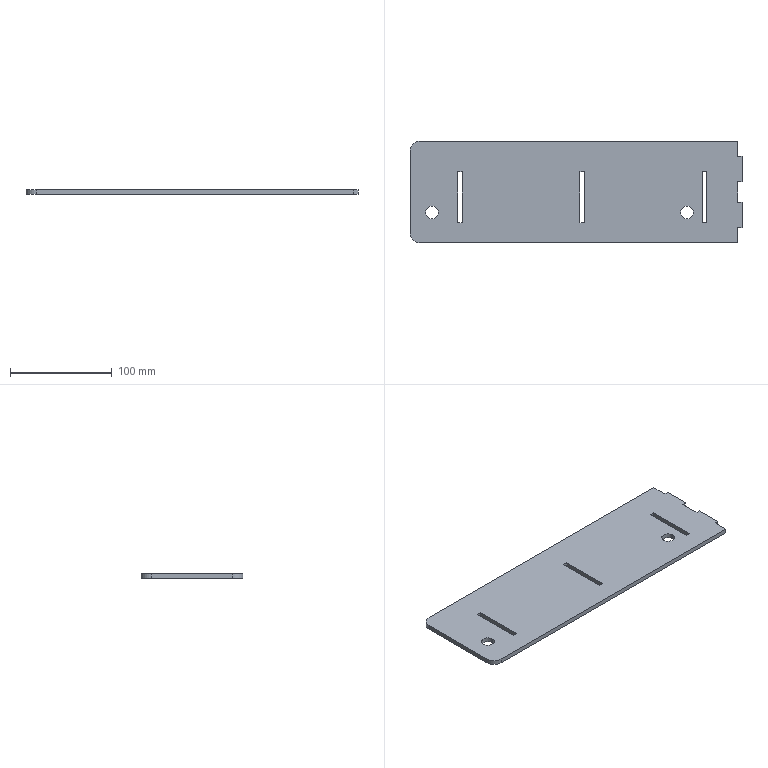Part | SolidWorks | features Fillet 1, FlatPattern 1, SMBaseFlange 1, SheetMetal 1 | 1 solid | 32 faces | box 325.679 x 100 x 4.5 mm | volume 141321 mm3 | plane 26 | cylinder 6 | commonest cylinder face diameters 12.5 x4 20 x2
STEP:
#1=CARTESIAN_POINT('',(173.75,-25.,4.5));
#2=VERTEX_POINT('',#1);
#3=CARTESIAN_POINT('',(186.25,-25.,4.5));
#4=VERTEX_POINT('',#3);
#5=CARTESIAN_POINT('',(180.,-25.,4.5));
#6=DIRECTION('',(0.,0.,1.));
#7=DIRECTION('',(1.,0.,0.));
#8=AXIS2_PLACEMENT_3D('',#5,#6,#7);
#9=CIRCLE('',#8,6.25);
#10=EDGE_CURVE('',#2,#4,#9,.T.);
#11=ORIENTED_EDGE('',*,*,#10,.T.);
#12=CARTESIAN_POINT('',(186.25,-25.,0.));
#13=VERTEX_POINT('',#12);
#14=CARTESIAN_POINT('',(186.25,-25.,4.5));
#15=DIRECTION('',(0.,0.,-1.));
#16=VECTOR('',#15,1000.);
#17=LINE('',#14,#16);
#18=EDGE_CURVE('',#4,#13,#17,.T.);
#19=ORIENTED_EDGE('',*,*,#18,.T.);
#20=CARTESIAN_POINT('',(173.75,-25.,0.));
#21=VERTEX_POINT('',#20);
#22=CARTESIAN_POINT('',(180.,-25.,0.));
#23=DIRECTION('',(0.,0.,1.));
#24=DIRECTION('',(1.,0.,0.));
#25=AXIS2_PLACEMENT_3D('',#22,#23,#24);
#26=CIRCLE('',#25,6.25);
#27=EDGE_CURVE('',#21,#13,#26,.T.);
#28=ORIENTED_EDGE('',*,*,#27,.F.);
#29=CARTESIAN_POINT('',(173.75,-25.,4.5));
#30=DIRECTION('',(0.,0.,-1.));
#31=VECTOR('',#30,1000.);
#32=LINE('',#29,#31);
#33=EDGE_CURVE('',#2,#21,#32,.T.);
#34=ORIENTED_EDGE('',*,*,#33,.F.);
#35=EDGE_LOOP('',(#11,#19,#28,#34));
#36=FACE_OUTER_BOUND('',#35,.T.);
#37=CARTESIAN_POINT('',(180.,-25.,4.5));
#38=DIRECTION('',(0.,0.,-1.));
#39=DIRECTION('',(-1.,0.,0.));
#40=AXIS2_PLACEMENT_3D('',#37,#38,#39);
#41=CYLINDRICAL_SURFACE('',#40,6.25);
#42=ADVANCED_FACE('',(#36),#41,.F.);
#43=CARTESIAN_POINT('',(-76.25,-25.,4.5));
#44=VERTEX_POINT('',#43);
#45=CARTESIAN_POINT('',(-63.75,-25.,4.5));
#46=VERTEX_POINT('',#45);
#47=CARTESIAN_POINT('',(-70.,-25.,4.5));
#48=DIRECTION('',(0.,0.,1.));
#49=DIRECTION('',(1.,0.,0.));
#50=AXIS2_PLACEMENT_3D('',#47,#48,#49);
#51=CIRCLE('',#50,6.25);
#52=EDGE_CURVE('',#44,#46,#51,.T.);
#53=ORIENTED_EDGE('',*,*,#52,.T.);
#54=CARTESIAN_POINT('',(-63.75,-25.,0.));
#55=VERTEX_POINT('',#54);
#56=CARTESIAN_POINT('',(-63.75,-25.,4.5));
#57=DIRECTION('',(0.,0.,-1.));
#58=VECTOR('',#57,1000.);
#59=LINE('',#56,#58);
#60=EDGE_CURVE('',#46,#55,#59,.T.);
#61=ORIENTED_EDGE('',*,*,#60,.T.);
#62=CARTESIAN_POINT('',(-76.25,-25.,0.));
#63=VERTEX_POINT('',#62);
#64=CARTESIAN_POINT('',(-70.,-25.,0.));
#65=DIRECTION('',(0.,0.,1.));
#66=DIRECTION('',(1.,0.,0.));
#67=AXIS2_PLACEMENT_3D('',#64,#65,#66);
#68=CIRCLE('',#67,6.25);
#69=EDGE_CURVE('',#63,#55,#68,.T.);
#70=ORIENTED_EDGE('',*,*,#69,.F.);
#71=CARTESIAN_POINT('',(-76.25,-25.,4.5));
#72=DIRECTION('',(0.,0.,-1.));
#73=VECTOR('',#72,1000.);
#74=LINE('',#71,#73);
#75=EDGE_CURVE('',#44,#63,#74,.T.);
#76=ORIENTED_EDGE('',*,*,#75,.F.);
#77=EDGE_LOOP('',(#53,#61,#70,#76));
#78=FACE_OUTER_BOUND('',#77,.T.);
#79=CARTESIAN_POINT('',(-70.,-25.,4.5));
#80=DIRECTION('',(0.,0.,-1.));
#81=DIRECTION('',(-1.,0.,0.));
#82=AXIS2_PLACEMENT_3D('',#79,#80,#81);
#83=CYLINDRICAL_SURFACE('',#82,6.25);
#84=ADVANCED_FACE('',(#78),#83,.F.);
#85=CARTESIAN_POINT('',(79.5,-35.,4.5));
#86=VERTEX_POINT('',#85);
#87=CARTESIAN_POINT('',(79.5,15.,4.5));
#88=VERTEX_POINT('',#87);
#89=CARTESIAN_POINT('',(79.5,-35.,4.5));
#90=DIRECTION('',(0.,1.,0.));
#91=VECTOR('',#90,1000.);
#92=LINE('',#89,#91);
#93=EDGE_CURVE('',#86,#88,#92,.T.);
#94=ORIENTED_EDGE('',*,*,#93,.F.);
#95=CARTESIAN_POINT('',(75.,-35.,4.5));
#96=VERTEX_POINT('',#95);
#97=CARTESIAN_POINT('',(79.5,-35.,4.5));
#98=DIRECTION('',(1.,0.,0.));
#99=VECTOR('',#98,1000.);
#100=LINE('',#97,#99);
#101=EDGE_CURVE('',#96,#86,#100,.T.);
#102=ORIENTED_EDGE('',*,*,#101,.F.);
#103=CARTESIAN_POINT('',(75.,15.,4.5));
#104=VERTEX_POINT('',#103);
#105=CARTESIAN_POINT('',(75.,-35.,4.5));
#106=DIRECTION('',(0.,-1.,0.));
#107=VECTOR('',#106,1000.);
#108=LINE('',#105,#107);
#109=EDGE_CURVE('',#104,#96,#108,.T.);
#110=ORIENTED_EDGE('',*,*,#109,.F.);
#111=CARTESIAN_POINT('',(79.5,15.,4.5));
#112=DIRECTION('',(-1.,0.,0.));
#113=VECTOR('',#112,1000.);
#114=LINE('',#111,#113);
#115=EDGE_CURVE('',#88,#104,#114,.T.);
#116=ORIENTED_EDGE('',*,*,#115,.F.);
#117=EDGE_LOOP('',(#94,#102,#110,#116));
#118=FACE_BOUND('',#117,.T.);
#119=CARTESIAN_POINT('',(-91.679,35.,4.5));
#120=VERTEX_POINT('',#119);
#121=CARTESIAN_POINT('',(-91.679,-45.,4.5));
#122=VERTEX_POINT('',#121);
#123=CARTESIAN_POINT('',(-91.679,-55.,4.5));
#124=DIRECTION('',(0.,-1.,0.));
#125=VECTOR('',#124,1000.);
#126=LINE('',#123,#125);
#127=EDGE_CURVE('',#120,#122,#126,.T.);
#128=ORIENTED_EDGE('',*,*,#127,.T.);
#129=CARTESIAN_POINT('',(-81.679,-55.,4.5));
#130=VERTEX_POINT('',#129);
#131=CARTESIAN_POINT('',(-81.679,-45.,4.5));
#132=DIRECTION('',(0.,0.,1.));
#133=DIRECTION('',(-1.,0.,0.));
#134=AXIS2_PLACEMENT_3D('',#131,#132,#133);
#135=CIRCLE('',#134,10.);
#136=EDGE_CURVE('',#122,#130,#135,.T.);
#137=ORIENTED_EDGE('',*,*,#136,.T.);
#138=CARTESIAN_POINT('',(230.,-55.,4.5));
#139=VERTEX_POINT('',#138);
#140=CARTESIAN_POINT('',(230.,-55.,4.5));
#141=DIRECTION('',(1.,0.,0.));
#142=VECTOR('',#141,1000.);
#143=LINE('',#140,#142);
#144=EDGE_CURVE('',#130,#139,#143,.T.);
#145=ORIENTED_EDGE('',*,*,#144,.T.);
#146=CARTESIAN_POINT('',(230.,-40.,4.5));
#147=VERTEX_POINT('',#146);
#148=CARTESIAN_POINT('',(230.,-40.,4.5));
#149=DIRECTION('',(0.,1.,0.));
#150=VECTOR('',#149,1000.);
#151=LINE('',#148,#150);
#152=EDGE_CURVE('',#139,#147,#151,.T.);
#153=ORIENTED_EDGE('',*,*,#152,.T.);
#154=CARTESIAN_POINT('',(234.,-40.,4.5));
#155=VERTEX_POINT('',#154);
#156=CARTESIAN_POINT('',(234.,-40.,4.5));
#157=DIRECTION('',(1.,0.,0.));
#158=VECTOR('',#157,1000.);
#159=LINE('',#156,#158);
#160=EDGE_CURVE('',#147,#155,#159,.T.);
#161=ORIENTED_EDGE('',*,*,#160,.T.);
#162=CARTESIAN_POINT('',(234.,-15.,4.5));
#163=VERTEX_POINT('',#162);
#164=CARTESIAN_POINT('',(234.,-15.,4.5));
#165=DIRECTION('',(0.,1.,0.));
#166=VECTOR('',#165,1000.);
#167=LINE('',#164,#166);
#168=EDGE_CURVE('',#155,#163,#167,.T.);
#169=ORIENTED_EDGE('',*,*,#168,.T.);
#170=CARTESIAN_POINT('',(230.,-15.,4.5));
#171=VERTEX_POINT('',#170);
#172=CARTESIAN_POINT('',(230.,-15.,4.5));
#173=DIRECTION('',(-1.,0.,0.));
#174=VECTOR('',#173,1000.);
#175=LINE('',#172,#174);
#176=EDGE_CURVE('',#163,#171,#175,.T.);
#177=ORIENTED_EDGE('',*,*,#176,.T.);
#178=CARTESIAN_POINT('',(230.,5.,4.5));
#179=VERTEX_POINT('',#178);
#180=CARTESIAN_POINT('',(230.,5.,4.5));
#181=DIRECTION('',(0.,1.,0.));
#182=VECTOR('',#181,1000.);
#183=LINE('',#180,#182);
#184=EDGE_CURVE('',#171,#179,#183,.T.);
#185=ORIENTED_EDGE('',*,*,#184,.T.);
#186=CARTESIAN_POINT('',(234.,5.,4.5));
#187=VERTEX_POINT('',#186);
#188=CARTESIAN_POINT('',(234.,5.,4.5));
#189=DIRECTION('',(1.,0.,0.));
#190=VECTOR('',#189,1000.);
#191=LINE('',#188,#190);
#192=EDGE_CURVE('',#179,#187,#191,.T.);
#193=ORIENTED_EDGE('',*,*,#192,.T.);
#194=CARTESIAN_POINT('',(234.,30.,4.5));
#195=VERTEX_POINT('',#194);
#196=CARTESIAN_POINT('',(234.,30.,4.5));
#197=DIRECTION('',(0.,1.,0.));
#198=VECTOR('',#197,1000.);
#199=LINE('',#196,#198);
#200=EDGE_CURVE('',#187,#195,#199,.T.);
#201=ORIENTED_EDGE('',*,*,#200,.T.);
#202=CARTESIAN_POINT('',(230.,30.,4.5));
#203=VERTEX_POINT('',#202);
#204=CARTESIAN_POINT('',(230.,30.,4.5));
#205=DIRECTION('',(-1.,0.,0.));
#206=VECTOR('',#205,1000.);
#207=LINE('',#204,#206);
#208=EDGE_CURVE('',#195,#203,#207,.T.);
#209=ORIENTED_EDGE('',*,*,#208,.T.);
#210=CARTESIAN_POINT('',(230.,45.,4.5));
#211=VERTEX_POINT('',#210);
#212=CARTESIAN_POINT('',(230.,45.,4.5));
#213=DIRECTION('',(0.,1.,0.));
#214=VECTOR('',#213,1000.);
#215=LINE('',#212,#214);
#216=EDGE_CURVE('',#203,#211,#215,.T.);
#217=ORIENTED_EDGE('',*,*,#216,.T.);
#218=CARTESIAN_POINT('',(-81.679,45.,4.5));
#219=VERTEX_POINT('',#218);
#220=CARTESIAN_POINT('',(-91.679,45.,4.5));
#221=DIRECTION('',(-1.,0.,0.));
#222=VECTOR('',#221,1000.);
#223=LINE('',#220,#222);
#224=EDGE_CURVE('',#211,#219,#223,.T.);
#225=ORIENTED_EDGE('',*,*,#224,.T.);
#226=CARTESIAN_POINT('',(-81.679,35.,4.5));
#227=DIRECTION('',(0.,0.,1.));
#228=DIRECTION('',(-1.,0.,0.));
#229=AXIS2_PLACEMENT_3D('',#226,#227,#228);
#230=CIRCLE('',#229,10.);
#231=EDGE_CURVE('',#219,#120,#230,.T.);
#232=ORIENTED_EDGE('',*,*,#231,.T.);
#233=EDGE_LOOP('',(#128,#137,#145,#153,#161,#169,#177,#185,#193,#201,#209,#217,#225,#232));
#234=FACE_OUTER_BOUND('',#233,.T.);
#235=CARTESIAN_POINT('',(-40.5,-35.,4.5));
#236=VERTEX_POINT('',#235);
#237=CARTESIAN_POINT('',(-40.5,15.,4.5));
#238=VERTEX_POINT('',#237);
#239=CARTESIAN_POINT('',(-40.5,-35.,4.5));
#240=DIRECTION('',(0.,1.,0.));
#241=VECTOR('',#240,1000.);
#242=LINE('',#239,#241);
#243=EDGE_CURVE('',#236,#238,#242,.T.);
#244=ORIENTED_EDGE('',*,*,#243,.F.);
#245=CARTESIAN_POINT('',(-45.,-35.,4.5));
#246=VERTEX_POINT('',#245);
#247=CARTESIAN_POINT('',(-40.5,-35.,4.5));
#248=DIRECTION('',(1.,0.,0.));
#249=VECTOR('',#248,1000.);
#250=LINE('',#247,#249);
#251=EDGE_CURVE('',#246,#236,#250,.T.);
#252=ORIENTED_EDGE('',*,*,#251,.F.);
#253=CARTESIAN_POINT('',(-45.,15.,4.5));
#254=VERTEX_POINT('',#253);
#255=CARTESIAN_POINT('',(-45.,-35.,4.5));
#256=DIRECTION('',(0.,-1.,0.));
#257=VECTOR('',#256,1000.);
#258=LINE('',#255,#257);
#259=EDGE_CURVE('',#254,#246,#258,.T.);
#260=ORIENTED_EDGE('',*,*,#259,.F.);
#261=CARTESIAN_POINT('',(-40.5,15.,4.5));
#262=DIRECTION('',(-1.,0.,0.));
#263=VECTOR('',#262,1000.);
#264=LINE('',#261,#263);
#265=EDGE_CURVE('',#238,#254,#264,.T.);
#266=ORIENTED_EDGE('',*,*,#265,.F.);
#267=EDGE_LOOP('',(#244,#252,#260,#266));
#268=FACE_BOUND('',#267,.T.);
#269=CARTESIAN_POINT('',(199.5,-35.,4.5));
#270=VERTEX_POINT('',#269);
#271=CARTESIAN_POINT('',(199.5,15.,4.5));
#272=VERTEX_POINT('',#271);
#273=CARTESIAN_POINT('',(199.5,-35.,4.5));
#274=DIRECTION('',(0.,1.,0.));
#275=VECTOR('',#274,1000.);
#276=LINE('',#273,#275);
#277=EDGE_CURVE('',#270,#272,#276,.T.);
#278=ORIENTED_EDGE('',*,*,#277,.F.);
#279=CARTESIAN_POINT('',(195.,-35.,4.5));
#280=VERTEX_POINT('',#279);
#281=CARTESIAN_POINT('',(199.5,-35.,4.5));
#282=DIRECTION('',(1.,0.,0.));
#283=VECTOR('',#282,1000.);
#284=LINE('',#281,#283);
#285=EDGE_CURVE('',#280,#270,#284,.T.);
#286=ORIENTED_EDGE('',*,*,#285,.F.);
#287=CARTESIAN_POINT('',(195.,15.,4.5));
#288=VERTEX_POINT('',#287);
#289=CARTESIAN_POINT('',(195.,-35.,4.5));
#290=DIRECTION('',(0.,-1.,0.));
#291=VECTOR('',#290,1000.);
#292=LINE('',#289,#291);
#293=EDGE_CURVE('',#288,#280,#292,.T.);
#294=ORIENTED_EDGE('',*,*,#293,.F.);
#295=CARTESIAN_POINT('',(199.5,15.,4.5));
#296=DIRECTION('',(-1.,0.,0.));
#297=VECTOR('',#296,1000.);
#298=LINE('',#295,#297);
#299=EDGE_CURVE('',#272,#288,#298,.T.);
#300=ORIENTED_EDGE('',*,*,#299,.F.);
#301=EDGE_LOOP('',(#278,#286,#294,#300));
#302=FACE_BOUND('',#301,.T.);
#303=ORIENTED_EDGE('',*,*,#52,.F.);
#304=CARTESIAN_POINT('',(-70.,-25.,4.5));
#305=DIRECTION('',(0.,0.,1.));
#306=DIRECTION('',(1.,0.,0.));
#307=AXIS2_PLACEMENT_3D('',#304,#305,#306);
#308=CIRCLE('',#307,6.25);
#309=EDGE_CURVE('',#46,#44,#308,.T.);
#310=ORIENTED_EDGE('',*,*,#309,.F.);
#311=EDGE_LOOP('',(#303,#310));
#312=FACE_BOUND('',#311,.T.);
#313=ORIENTED_EDGE('',*,*,#10,.F.);
#314=CARTESIAN_POINT('',(180.,-25.,4.5));
#315=DIRECTION('',(0.,0.,1.));
#316=DIRECTION('',(1.,0.,0.));
#317=AXIS2_PLACEMENT_3D('',#314,#315,#316);
#318=CIRCLE('',#317,6.25);
#319=EDGE_CURVE('',#4,#2,#318,.T.);
#320=ORIENTED_EDGE('',*,*,#319,.F.);
#321=EDGE_LOOP('',(#313,#320));
#322=FACE_BOUND('',#321,.T.);
#323=CARTESIAN_POINT('',(0.,0.,4.5));
#324=DIRECTION('',(0.,0.,-1.));
#325=DIRECTION('',(-1.,0.,0.));
#326=AXIS2_PLACEMENT_3D('',#323,#324,#325);
#327=PLANE('',#326);
#328=ADVANCED_FACE('',(#118,#234,#268,#302,#312,#322),#327,.F.);
#329=ORIENTED_EDGE('',*,*,#69,.T.);
#330=CARTESIAN_POINT('',(-70.,-25.,0.));
#331=DIRECTION('',(0.,0.,1.));
#332=DIRECTION('',(1.,0.,0.));
#333=AXIS2_PLACEMENT_3D('',#330,#331,#332);
#334=CIRCLE('',#333,6.25);
#335=EDGE_CURVE('',#55,#63,#334,.T.);
#336=ORIENTED_EDGE('',*,*,#335,.T.);
#337=EDGE_LOOP('',(#329,#336));
#338=FACE_BOUND('',#337,.T.);
#339=CARTESIAN_POINT('',(-81.679,-55.,0.));
#340=VERTEX_POINT('',#339);
#341=CARTESIAN_POINT('',(230.,-55.,0.));
#342=VERTEX_POINT('',#341);
#343=CARTESIAN_POINT('',(230.,-55.,0.));
#344=DIRECTION('',(1.,0.,0.));
#345=VECTOR('',#344,1000.);
#346=LINE('',#343,#345);
#347=EDGE_CURVE('',#340,#342,#346,.T.);
#348=ORIENTED_EDGE('',*,*,#347,.F.);
#349=CARTESIAN_POINT('',(-91.679,-45.,0.));
#350=VERTEX_POINT('',#349);
#351=CARTESIAN_POINT('',(-81.679,-45.,0.));
#352=DIRECTION('',(0.,0.,-1.));
#353=DIRECTION('',(-1.,0.,0.));
#354=AXIS2_PLACEMENT_3D('',#351,#352,#353);
#355=CIRCLE('',#354,10.);
#356=EDGE_CURVE('',#340,#350,#355,.T.);
#357=ORIENTED_EDGE('',*,*,#356,.T.);
#358=CARTESIAN_POINT('',(-91.679,35.,0.));
#359=VERTEX_POINT('',#358);
#360=CARTESIAN_POINT('',(-91.679,-55.,0.));
#361=DIRECTION('',(0.,-1.,0.));
#362=VECTOR('',#361,1000.);
#363=LINE('',#360,#362);
#364=EDGE_CURVE('',#359,#350,#363,.T.);
#365=ORIENTED_EDGE('',*,*,#364,.F.);
#366=CARTESIAN_POINT('',(-81.679,45.,0.));
#367=VERTEX_POINT('',#366);
#368=CARTESIAN_POINT('',(-81.679,35.,0.));
#369=DIRECTION('',(0.,0.,-1.));
#370=DIRECTION('',(-1.,0.,0.));
#371=AXIS2_PLACEMENT_3D('',#368,#369,#370);
#372=CIRCLE('',#371,10.);
#373=EDGE_CURVE('',#359,#367,#372,.T.);
#374=ORIENTED_EDGE('',*,*,#373,.T.);
#375=CARTESIAN_POINT('',(230.,45.,0.));
#376=VERTEX_POINT('',#375);
#377=CARTESIAN_POINT('',(-91.679,45.,0.));
#378=DIRECTION('',(-1.,0.,0.));
#379=VECTOR('',#378,1000.);
#380=LINE('',#377,#379);
#381=EDGE_CURVE('',#376,#367,#380,.T.);
#382=ORIENTED_EDGE('',*,*,#381,.F.);
#383=CARTESIAN_POINT('',(230.,30.,0.));
#384=VERTEX_POINT('',#383);
#385=CARTESIAN_POINT('',(230.,45.,0.));
#386=DIRECTION('',(0.,1.,0.));
#387=VECTOR('',#386,1000.);
#388=LINE('',#385,#387);
#389=EDGE_CURVE('',#384,#376,#388,.T.);
#390=ORIENTED_EDGE('',*,*,#389,.F.);
#391=CARTESIAN_POINT('',(234.,30.,0.));
#392=VERTEX_POINT('',#391);
#393=CARTESIAN_POINT('',(230.,30.,0.));
#394=DIRECTION('',(-1.,0.,0.));
#395=VECTOR('',#394,1000.);
#396=LINE('',#393,#395);
#397=EDGE_CURVE('',#392,#384,#396,.T.);
#398=ORIENTED_EDGE('',*,*,#397,.F.);
#399=CARTESIAN_POINT('',(234.,5.,0.));
#400=VERTEX_POINT('',#399);
#401=CARTESIAN_POINT('',(234.,30.,0.));
#402=DIRECTION('',(0.,1.,0.));
#403=VECTOR('',#402,1000.);
#404=LINE('',#401,#403);
#405=EDGE_CURVE('',#400,#392,#404,.T.);
#406=ORIENTED_EDGE('',*,*,#405,.F.);
#407=CARTESIAN_POINT('',(230.,5.,0.));
#408=VERTEX_POINT('',#407);
#409=CARTESIAN_POINT('',(234.,5.,0.));
#410=DIRECTION('',(1.,0.,0.));
#411=VECTOR('',#410,1000.);
#412=LINE('',#409,#411);
#413=EDGE_CURVE('',#408,#400,#412,.T.);
#414=ORIENTED_EDGE('',*,*,#413,.F.);
#415=CARTESIAN_POINT('',(230.,-15.,0.));
#416=VERTEX_POINT('',#415);
#417=CARTESIAN_POINT('',(230.,5.,0.));
#418=DIRECTION('',(0.,1.,0.));
#419=VECTOR('',#418,1000.);
#420=LINE('',#417,#419);
#421=EDGE_CURVE('',#416,#408,#420,.T.);
#422=ORIENTED_EDGE('',*,*,#421,.F.);
#423=CARTESIAN_POINT('',(234.,-15.,0.));
#424=VERTEX_POINT('',#423);
#425=CARTESIAN_POINT('',(230.,-15.,0.));
#426=DIRECTION('',(-1.,0.,0.));
#427=VECTOR('',#426,1000.);
#428=LINE('',#425,#427);
#429=EDGE_CURVE('',#424,#416,#428,.T.);
#430=ORIENTED_EDGE('',*,*,#429,.F.);
#431=CARTESIAN_POINT('',(234.,-40.,0.));
#432=VERTEX_POINT('',#431);
#433=CARTESIAN_POINT('',(234.,-15.,0.));
#434=DIRECTION('',(0.,1.,0.));
#435=VECTOR('',#434,1000.);
#436=LINE('',#433,#435);
#437=EDGE_CURVE('',#432,#424,#436,.T.);
#438=ORIENTED_EDGE('',*,*,#437,.F.);
#439=CARTESIAN_POINT('',(230.,-40.,0.));
#440=VERTEX_POINT('',#439);
#441=CARTESIAN_POINT('',(234.,-40.,0.));
#442=DIRECTION('',(1.,0.,0.));
#443=VECTOR('',#442,1000.);
#444=LINE('',#441,#443);
#445=EDGE_CURVE('',#440,#432,#444,.T.);
#446=ORIENTED_EDGE('',*,*,#445,.F.);
#447=CARTESIAN_POINT('',(230.,-40.,0.));
#448=DIRECTION('',(0.,1.,0.));
#449=VECTOR('',#448,1000.);
#450=LINE('',#447,#449);
#451=EDGE_CURVE('',#342,#440,#450,.T.);
#452=ORIENTED_EDGE('',*,*,#451,.F.);
#453=EDGE_LOOP('',(#348,#357,#365,#374,#382,#390,#398,#406,#414,#422,#430,#438,#446,#452));
#454=FACE_OUTER_BOUND('',#453,.T.);
#455=CARTESIAN_POINT('',(-45.,-35.,0.));
#456=VERTEX_POINT('',#455);
#457=CARTESIAN_POINT('',(-40.5,-35.,0.));
#458=VERTEX_POINT('',#457);
#459=CARTESIAN_POINT('',(-40.5,-35.,0.));
#460=DIRECTION('',(1.,0.,0.));
#461=VECTOR('',#460,1000.);
#462=LINE('',#459,#461);
#463=EDGE_CURVE('',#456,#458,#462,.T.);
#464=ORIENTED_EDGE('',*,*,#463,.T.);
#465=CARTESIAN_POINT('',(-40.5,15.,0.));
#466=VERTEX_POINT('',#465);
#467=CARTESIAN_POINT('',(-40.5,-35.,0.));
#468=DIRECTION('',(0.,1.,0.));
#469=VECTOR('',#468,1000.);
#470=LINE('',#467,#469);
#471=EDGE_CURVE('',#458,#466,#470,.T.);
#472=ORIENTED_EDGE('',*,*,#471,.T.);
#473=CARTESIAN_POINT('',(-45.,15.,0.));
#474=VERTEX_POINT('',#473);
#475=CARTESIAN_POINT('',(-40.5,15.,0.));
#476=DIRECTION('',(-1.,0.,0.));
#477=VECTOR('',#476,1000.);
#478=LINE('',#475,#477);
#479=EDGE_CURVE('',#466,#474,#478,.T.);
#480=ORIENTED_EDGE('',*,*,#479,.T.);
#481=CARTESIAN_POINT('',(-45.,-35.,0.));
#482=DIRECTION('',(0.,-1.,0.));
#483=VECTOR('',#482,1000.);
#484=LINE('',#481,#483);
#485=EDGE_CURVE('',#474,#456,#484,.T.);
#486=ORIENTED_EDGE('',*,*,#485,.T.);
#487=EDGE_LOOP('',(#464,#472,#480,#486));
#488=FACE_BOUND('',#487,.T.);
#489=CARTESIAN_POINT('',(75.,-35.,0.));
#490=VERTEX_POINT('',#489);
#491=CARTESIAN_POINT('',(79.5,-35.,0.));
#492=VERTEX_POINT('',#491);
#493=CARTESIAN_POINT('',(79.5,-35.,0.));
#494=DIRECTION('',(1.,0.,0.));
#495=VECTOR('',#494,1000.);
#496=LINE('',#493,#495);
#497=EDGE_CURVE('',#490,#492,#496,.T.);
#498=ORIENTED_EDGE('',*,*,#497,.T.);
#499=CARTESIAN_POINT('',(79.5,15.,0.));
#500=VERTEX_POINT('',#499);
#501=CARTESIAN_POINT('',(79.5,-35.,0.));
#502=DIRECTION('',(0.,1.,0.));
#503=VECTOR('',#502,1000.);
#504=LINE('',#501,#503);
#505=EDGE_CURVE('',#492,#500,#504,.T.);
#506=ORIENTED_EDGE('',*,*,#505,.T.);
#507=CARTESIAN_POINT('',(75.,15.,0.));
#508=VERTEX_POINT('',#507);
#509=CARTESIAN_POINT('',(79.5,15.,0.));
#510=DIRECTION('',(-1.,0.,0.));
#511=VECTOR('',#510,1000.);
#512=LINE('',#509,#511);
#513=EDGE_CURVE('',#500,#508,#512,.T.);
#514=ORIENTED_EDGE('',*,*,#513,.T.);
#515=CARTESIAN_POINT('',(75.,-35.,0.));
#516=DIRECTION('',(0.,-1.,0.));
#517=VECTOR('',#516,1000.);
#518=LINE('',#515,#517);
#519=EDGE_CURVE('',#508,#490,#518,.T.);
#520=ORIENTED_EDGE('',*,*,#519,.T.);
#521=EDGE_LOOP('',(#498,#506,#514,#520));
#522=FACE_BOUND('',#521,.T.);
#523=CARTESIAN_POINT('',(195.,-35.,0.));
#524=VERTEX_POINT('',#523);
#525=CARTESIAN_POINT('',(199.5,-35.,0.));
#526=VERTEX_POINT('',#525);
#527=CARTESIAN_POINT('',(199.5,-35.,0.));
#528=DIRECTION('',(1.,0.,0.));
#529=VECTOR('',#528,1000.);
#530=LINE('',#527,#529);
#531=EDGE_CURVE('',#524,#526,#530,.T.);
#532=ORIENTED_EDGE('',*,*,#531,.T.);
#533=CARTESIAN_POINT('',(199.5,15.,0.));
#534=VERTEX_POINT('',#533);
#535=CARTESIAN_POINT('',(199.5,-35.,0.));
#536=DIRECTION('',(0.,1.,0.));
#537=VECTOR('',#536,1000.);
#538=LINE('',#535,#537);
#539=EDGE_CURVE('',#526,#534,#538,.T.);
#540=ORIENTED_EDGE('',*,*,#539,.T.);
#541=CARTESIAN_POINT('',(195.,15.,0.));
#542=VERTEX_POINT('',#541);
#543=CARTESIAN_POINT('',(199.5,15.,0.));
#544=DIRECTION('',(-1.,0.,0.));
#545=VECTOR('',#544,1000.);
#546=LINE('',#543,#545);
#547=EDGE_CURVE('',#534,#542,#546,.T.);
#548=ORIENTED_EDGE('',*,*,#547,.T.);
#549=CARTESIAN_POINT('',(195.,-35.,0.));
#550=DIRECTION('',(0.,-1.,0.));
#551=VECTOR('',#550,1000.);
#552=LINE('',#549,#551);
#553=EDGE_CURVE('',#542,#524,#552,.T.);
#554=ORIENTED_EDGE('',*,*,#553,.T.);
#555=EDGE_LOOP('',(#532,#540,#548,#554));
#556=FACE_BOUND('',#555,.T.);
#557=ORIENTED_EDGE('',*,*,#27,.T.);
#558=CARTESIAN_POINT('',(180.,-25.,0.));
#559=DIRECTION('',(0.,0.,1.));
#560=DIRECTION('',(1.,0.,0.));
#561=AXIS2_PLACEMENT_3D('',#558,#559,#560);
#562=CIRCLE('',#561,6.25);
#563=EDGE_CURVE('',#13,#21,#562,.T.);
#564=ORIENTED_EDGE('',*,*,#563,.T.);
#565=EDGE_LOOP('',(#557,#564));
#566=FACE_BOUND('',#565,.T.);
#567=CARTESIAN_POINT('',(0.,0.,0.));
#568=DIRECTION('',(0.,0.,-1.));
#569=DIRECTION('',(-1.,0.,0.));
#570=AXIS2_PLACEMENT_3D('',#567,#568,#569);
#571=PLANE('',#570);
#572=ADVANCED_FACE('',(#338,#454,#488,#522,#556,#566),#571,.T.);
#573=ORIENTED_EDGE('',*,*,#451,.T.);
#574=CARTESIAN_POINT('',(230.,-40.,4.5));
#575=DIRECTION('',(0.,0.,-1.));
#576=VECTOR('',#575,1000.);
#577=LINE('',#574,#576);
#578=EDGE_CURVE('',#147,#440,#577,.T.);
#579=ORIENTED_EDGE('',*,*,#578,.F.);
#580=ORIENTED_EDGE('',*,*,#152,.F.);
#581=CARTESIAN_POINT('',(230.,-55.,4.5));
#582=DIRECTION('',(0.,0.,-1.));
#583=VECTOR('',#582,1000.);
#584=LINE('',#581,#583);
#585=EDGE_CURVE('',#139,#342,#584,.T.);
#586=ORIENTED_EDGE('',*,*,#585,.T.);
#587=EDGE_LOOP('',(#573,#579,#580,#586));
#588=FACE_OUTER_BOUND('',#587,.T.);
#589=CARTESIAN_POINT('',(230.,-40.,4.5));
#590=DIRECTION('',(-1.,0.,0.));
#591=DIRECTION('',(0.,0.,1.));
#592=AXIS2_PLACEMENT_3D('',#589,#590,#591);
#593=PLANE('',#592);
#594=ADVANCED_FACE('',(#588),#593,.F.);
#595=ORIENTED_EDGE('',*,*,#445,.T.);
#596=CARTESIAN_POINT('',(234.,-40.,4.5));
#597=DIRECTION('',(0.,0.,-1.));
#598=VECTOR('',#597,1000.);
#599=LINE('',#596,#598);
#600=EDGE_CURVE('',#155,#432,#599,.T.);
#601=ORIENTED_EDGE('',*,*,#600,.F.);
#602=ORIENTED_EDGE('',*,*,#160,.F.);
#603=ORIENTED_EDGE('',*,*,#578,.T.);
#604=EDGE_LOOP('',(#595,#601,#602,#603));
#605=FACE_OUTER_BOUND('',#604,.T.);
#606=CARTESIAN_POINT('',(234.,-40.,4.5));
#607=DIRECTION('',(0.,1.,0.));
#608=DIRECTION('',(0.,0.,1.));
#609=AXIS2_PLACEMENT_3D('',#606,#607,#608);
#610=PLANE('',#609);
#611=ADVANCED_FACE('',(#605),#610,.F.);
#612=ORIENTED_EDGE('',*,*,#437,.T.);
#613=CARTESIAN_POINT('',(234.,-15.,4.5));
#614=DIRECTION('',(0.,0.,-1.));
#615=VECTOR('',#614,1000.);
#616=LINE('',#613,#615);
#617=EDGE_CURVE('',#163,#424,#616,.T.);
#618=ORIENTED_EDGE('',*,*,#617,.F.);
#619=ORIENTED_EDGE('',*,*,#168,.F.);
#620=ORIENTED_EDGE('',*,*,#600,.T.);
#621=EDGE_LOOP('',(#612,#618,#619,#620));
#622=FACE_OUTER_BOUND('',#621,.T.);
#623=CARTESIAN_POINT('',(234.,-15.,4.5));
#624=DIRECTION('',(-1.,0.,0.));
#625=DIRECTION('',(0.,0.,1.));
#626=AXIS2_PLACEMENT_3D('',#623,#624,#625);
#627=PLANE('',#626);
#628=ADVANCED_FACE('',(#622),#627,.F.);
#629=ORIENTED_EDGE('',*,*,#429,.T.);
#630=CARTESIAN_POINT('',(230.,-15.,4.5));
#631=DIRECTION('',(0.,0.,-1.));
#632=VECTOR('',#631,1000.);
#633=LINE('',#630,#632);
#634=EDGE_CURVE('',#171,#416,#633,.T.);
#635=ORIENTED_EDGE('',*,*,#634,.F.);
#636=ORIENTED_EDGE('',*,*,#176,.F.);
#637=ORIENTED_EDGE('',*,*,#617,.T.);
#638=EDGE_LOOP('',(#629,#635,#636,#637));
#639=FACE_OUTER_BOUND('',#638,.T.);
#640=CARTESIAN_POINT('',(230.,-15.,4.5));
#641=DIRECTION('',(0.,-1.,0.));
#642=DIRECTION('',(1.,0.,0.));
#643=AXIS2_PLACEMENT_3D('',#640,#641,#642);
#644=PLANE('',#643);
#645=ADVANCED_FACE('',(#639),#644,.F.);
#646=ORIENTED_EDGE('',*,*,#421,.T.);
#647=CARTESIAN_POINT('',(230.,5.,4.5));
#648=DIRECTION('',(0.,0.,-1.));
#649=VECTOR('',#648,1000.);
#650=LINE('',#647,#649);
#651=EDGE_CURVE('',#179,#408,#650,.T.);
#652=ORIENTED_EDGE('',*,*,#651,.F.);
#653=ORIENTED_EDGE('',*,*,#184,.F.);
#654=ORIENTED_EDGE('',*,*,#634,.T.);
#655=EDGE_LOOP('',(#646,#652,#653,#654));
#656=FACE_OUTER_BOUND('',#655,.T.);
#657=CARTESIAN_POINT('',(230.,5.,4.5));
#658=DIRECTION('',(-1.,0.,0.));
#659=DIRECTION('',(0.,0.,1.));
#660=AXIS2_PLACEMENT_3D('',#657,#658,#659);
#661=PLANE('',#660);
#662=ADVANCED_FACE('',(#656),#661,.F.);
#663=ORIENTED_EDGE('',*,*,#413,.T.);
#664=CARTESIAN_POINT('',(234.,5.,4.5));
#665=DIRECTION('',(0.,0.,-1.));
#666=VECTOR('',#665,1000.);
#667=LINE('',#664,#666);
#668=EDGE_CURVE('',#187,#400,#667,.T.);
#669=ORIENTED_EDGE('',*,*,#668,.F.);
#670=ORIENTED_EDGE('',*,*,#192,.F.);
#671=ORIENTED_EDGE('',*,*,#651,.T.);
#672=EDGE_LOOP('',(#663,#669,#670,#671));
#673=FACE_OUTER_BOUND('',#672,.T.);
#674=CARTESIAN_POINT('',(234.,5.,4.5));
#675=DIRECTION('',(0.,1.,0.));
#676=DIRECTION('',(-1.,0.,0.));
#677=AXIS2_PLACEMENT_3D('',#674,#675,#676);
#678=PLANE('',#677);
#679=ADVANCED_FACE('',(#673),#678,.F.);
#680=ORIENTED_EDGE('',*,*,#405,.T.);
#681=CARTESIAN_POINT('',(234.,30.,4.5));
#682=DIRECTION('',(0.,0.,-1.));
#683=VECTOR('',#682,1000.);
#684=LINE('',#681,#683);
#685=EDGE_CURVE('',#195,#392,#684,.T.);
#686=ORIENTED_EDGE('',*,*,#685,.F.);
#687=ORIENTED_EDGE('',*,*,#200,.F.);
#688=ORIENTED_EDGE('',*,*,#668,.T.);
#689=EDGE_LOOP('',(#680,#686,#687,#688));
#690=FACE_OUTER_BOUND('',#689,.T.);
#691=CARTESIAN_POINT('',(234.,30.,4.5));
#692=DIRECTION('',(-1.,0.,0.));
#693=DIRECTION('',(0.,0.,1.));
#694=AXIS2_PLACEMENT_3D('',#691,#692,#693);
#695=PLANE('',#694);
#696=ADVANCED_FACE('',(#690),#695,.F.);
#697=ORIENTED_EDGE('',*,*,#397,.T.);
#698=CARTESIAN_POINT('',(230.,30.,4.5));
#699=DIRECTION('',(0.,0.,-1.));
#700=VECTOR('',#699,1000.);
#701=LINE('',#698,#700);
#702=EDGE_CURVE('',#203,#384,#701,.T.);
#703=ORIENTED_EDGE('',*,*,#702,.F.);
#704=ORIENTED_EDGE('',*,*,#208,.F.);
#705=ORIENTED_EDGE('',*,*,#685,.T.);
#706=EDGE_LOOP('',(#697,#703,#704,#705));
#707=FACE_OUTER_BOUND('',#706,.T.);
#708=CARTESIAN_POINT('',(230.,30.,4.5));
#709=DIRECTION('',(0.,-1.,0.));
#710=DIRECTION('',(0.,0.,-1.));
#711=AXIS2_PLACEMENT_3D('',#708,#709,#710);
#712=PLANE('',#711);
#713=ADVANCED_FACE('',(#707),#712,.F.);
#714=ORIENTED_EDGE('',*,*,#389,.T.);
#715=CARTESIAN_POINT('',(230.,45.,4.5));
#716=DIRECTION('',(0.,0.,-1.));
#717=VECTOR('',#716,1000.);
#718=LINE('',#715,#717);
#719=EDGE_CURVE('',#211,#376,#718,.T.);
#720=ORIENTED_EDGE('',*,*,#719,.F.);
#721=ORIENTED_EDGE('',*,*,#216,.F.);
#722=ORIENTED_EDGE('',*,*,#702,.T.);
#723=EDGE_LOOP('',(#714,#720,#721,#722));
#724=FACE_OUTER_BOUND('',#723,.T.);
#725=CARTESIAN_POINT('',(230.,45.,4.5));
#726=DIRECTION('',(-1.,0.,0.));
#727=DIRECTION('',(0.,-1.,0.));
#728=AXIS2_PLACEMENT_3D('',#725,#726,#727);
#729=PLANE('',#728);
#730=ADVANCED_FACE('',(#724),#729,.F.);
#731=ORIENTED_EDGE('',*,*,#381,.T.);
#732=CARTESIAN_POINT('',(-81.679,45.,4.5));
#733=DIRECTION('',(0.,0.,1.));
#734=VECTOR('',#733,1000.);
#735=LINE('',#732,#734);
#736=EDGE_CURVE('',#367,#219,#735,.T.);
#737=ORIENTED_EDGE('',*,*,#736,.T.);
#738=ORIENTED_EDGE('',*,*,#224,.F.);
#739=ORIENTED_EDGE('',*,*,#719,.T.);
#740=EDGE_LOOP('',(#731,#737,#738,#739));
#741=FACE_OUTER_BOUND('',#740,.T.);
#742=CARTESIAN_POINT('',(-91.679,45.,4.5));
#743=DIRECTION('',(0.,-1.,0.));
#744=DIRECTION('',(0.,0.,-1.));
#745=AXIS2_PLACEMENT_3D('',#742,#743,#744);
#746=PLANE('',#745);
#747=ADVANCED_FACE('',(#741),#746,.F.);
#748=ORIENTED_EDGE('',*,*,#364,.T.);
#749=CARTESIAN_POINT('',(-91.679,-45.,4.5));
#750=DIRECTION('',(0.,0.,1.));
#751=VECTOR('',#750,1000.);
#752=LINE('',#749,#751);
#753=EDGE_CURVE('',#350,#122,#752,.T.);
#754=ORIENTED_EDGE('',*,*,#753,.T.);
#755=ORIENTED_EDGE('',*,*,#127,.F.);
#756=CARTESIAN_POINT('',(-91.679,35.,4.5));
#757=DIRECTION('',(0.,0.,-1.));
#758=VECTOR('',#757,1000.);
#759=LINE('',#756,#758);
#760=EDGE_CURVE('',#120,#359,#759,.T.);
#761=ORIENTED_EDGE('',*,*,#760,.T.);
#762=EDGE_LOOP('',(#748,#754,#755,#761));
#763=FACE_OUTER_BOUND('',#762,.T.);
#764=CARTESIAN_POINT('',(-91.679,-55.,4.5));
#765=DIRECTION('',(1.,0.,0.));
#766=DIRECTION('',(0.,1.,0.));
#767=AXIS2_PLACEMENT_3D('',#764,#765,#766);
#768=PLANE('',#767);
#769=ADVANCED_FACE('',(#763),#768,.F.);
#770=ORIENTED_EDGE('',*,*,#144,.F.);
#771=CARTESIAN_POINT('',(-81.679,-55.,4.5));
#772=DIRECTION('',(0.,0.,-1.));
#773=VECTOR('',#772,1000.);
#774=LINE('',#771,#773);
#775=EDGE_CURVE('',#130,#340,#774,.T.);
#776=ORIENTED_EDGE('',*,*,#775,.T.);
#777=ORIENTED_EDGE('',*,*,#347,.T.);
#778=ORIENTED_EDGE('',*,*,#585,.F.);
#779=EDGE_LOOP('',(#770,#776,#777,#778));
#780=FACE_OUTER_BOUND('',#779,.T.);
#781=CARTESIAN_POINT('',(230.,-55.,4.5));
#782=DIRECTION('',(0.,1.,0.));
#783=DIRECTION('',(-1.,0.,0.));
#784=AXIS2_PLACEMENT_3D('',#781,#782,#783);
#785=PLANE('',#784);
#786=ADVANCED_FACE('',(#780),#785,.F.);
#787=ORIENTED_EDGE('',*,*,#471,.F.);
#788=CARTESIAN_POINT('',(-40.5,-35.,4.5));
#789=DIRECTION('',(0.,0.,-1.));
#790=VECTOR('',#789,1000.);
#791=LINE('',#788,#790);
#792=EDGE_CURVE('',#236,#458,#791,.T.);
#793=ORIENTED_EDGE('',*,*,#792,.F.);
#794=ORIENTED_EDGE('',*,*,#243,.T.);
#795=CARTESIAN_POINT('',(-40.5,15.,4.5));
#796=DIRECTION('',(0.,0.,-1.));
#797=VECTOR('',#796,1000.);
#798=LINE('',#795,#797);
#799=EDGE_CURVE('',#238,#466,#798,.T.);
#800=ORIENTED_EDGE('',*,*,#799,.T.);
#801=EDGE_LOOP('',(#787,#793,#794,#800));
#802=FACE_OUTER_BOUND('',#801,.T.);
#803=CARTESIAN_POINT('',(-40.5,-35.,4.5));
#804=DIRECTION('',(-1.,0.,0.));
#805=DIRECTION('',(0.,0.,1.));
#806=AXIS2_PLACEMENT_3D('',#803,#804,#805);
#807=PLANE('',#806);
#808=ADVANCED_FACE('',(#802),#807,.T.);
#809=ORIENTED_EDGE('',*,*,#479,.F.);
#810=ORIENTED_EDGE('',*,*,#799,.F.);
#811=ORIENTED_EDGE('',*,*,#265,.T.);
#812=CARTESIAN_POINT('',(-45.,15.,4.5));
#813=DIRECTION('',(0.,0.,-1.));
#814=VECTOR('',#813,1000.);
#815=LINE('',#812,#814);
#816=EDGE_CURVE('',#254,#474,#815,.T.);
#817=ORIENTED_EDGE('',*,*,#816,.T.);
#818=EDGE_LOOP('',(#809,#810,#811,#817));
#819=FACE_OUTER_BOUND('',#818,.T.);
#820=CARTESIAN_POINT('',(-40.5,15.,4.5));
#821=DIRECTION('',(0.,-1.,0.));
#822=DIRECTION('',(0.,0.,-1.));
#823=AXIS2_PLACEMENT_3D('',#820,#821,#822);
#824=PLANE('',#823);
#825=ADVANCED_FACE('',(#819),#824,.T.);
#826=ORIENTED_EDGE('',*,*,#485,.F.);
#827=ORIENTED_EDGE('',*,*,#816,.F.);
#828=ORIENTED_EDGE('',*,*,#259,.T.);
#829=CARTESIAN_POINT('',(-45.,-35.,4.5));
#830=DIRECTION('',(0.,0.,-1.));
#831=VECTOR('',#830,1000.);
#832=LINE('',#829,#831);
#833=EDGE_CURVE('',#246,#456,#832,.T.);
#834=ORIENTED_EDGE('',*,*,#833,.T.);
#835=EDGE_LOOP('',(#826,#827,#828,#834));
#836=FACE_OUTER_BOUND('',#835,.T.);
#837=CARTESIAN_POINT('',(-45.,-35.,4.5));
#838=DIRECTION('',(1.,0.,0.));
#839=DIRECTION('',(0.,0.,-1.));
#840=AXIS2_PLACEMENT_3D('',#837,#838,#839);
#841=PLANE('',#840);
#842=ADVANCED_FACE('',(#836),#841,.T.);
#843=ORIENTED_EDGE('',*,*,#463,.F.);
#844=ORIENTED_EDGE('',*,*,#833,.F.);
#845=ORIENTED_EDGE('',*,*,#251,.T.);
#846=ORIENTED_EDGE('',*,*,#792,.T.);
#847=EDGE_LOOP('',(#843,#844,#845,#846));
#848=FACE_OUTER_BOUND('',#847,.T.);
#849=CARTESIAN_POINT('',(-40.5,-35.,4.5));
#850=DIRECTION('',(0.,1.,0.));
#851=DIRECTION('',(0.,0.,1.));
#852=AXIS2_PLACEMENT_3D('',#849,#850,#851);
#853=PLANE('',#852);
#854=ADVANCED_FACE('',(#848),#853,.T.);
#855=ORIENTED_EDGE('',*,*,#505,.F.);
#856=CARTESIAN_POINT('',(79.5,-35.,4.5));
#857=DIRECTION('',(0.,0.,-1.));
#858=VECTOR('',#857,1000.);
#859=LINE('',#856,#858);
#860=EDGE_CURVE('',#86,#492,#859,.T.);
#861=ORIENTED_EDGE('',*,*,#860,.F.);
#862=ORIENTED_EDGE('',*,*,#93,.T.);
#863=CARTESIAN_POINT('',(79.5,15.,4.5));
#864=DIRECTION('',(0.,0.,-1.));
#865=VECTOR('',#864,1000.);
#866=LINE('',#863,#865);
#867=EDGE_CURVE('',#88,#500,#866,.T.);
#868=ORIENTED_EDGE('',*,*,#867,.T.);
#869=EDGE_LOOP('',(#855,#861,#862,#868));
#870=FACE_OUTER_BOUND('',#869,.T.);
#871=CARTESIAN_POINT('',(79.5,-35.,4.5));
#872=DIRECTION('',(-1.,0.,0.));
#873=DIRECTION('',(0.,0.,1.));
#874=AXIS2_PLACEMENT_3D('',#871,#872,#873);
#875=PLANE('',#874);
#876=ADVANCED_FACE('',(#870),#875,.T.);
#877=ORIENTED_EDGE('',*,*,#513,.F.);
#878=ORIENTED_EDGE('',*,*,#867,.F.);
#879=ORIENTED_EDGE('',*,*,#115,.T.);
#880=CARTESIAN_POINT('',(75.,15.,4.5));
#881=DIRECTION('',(0.,0.,-1.));
#882=VECTOR('',#881,1000.);
#883=LINE('',#880,#882);
#884=EDGE_CURVE('',#104,#508,#883,.T.);
#885=ORIENTED_EDGE('',*,*,#884,.T.);
#886=EDGE_LOOP('',(#877,#878,#879,#885));
#887=FACE_OUTER_BOUND('',#886,.T.);
#888=CARTESIAN_POINT('',(79.5,15.,4.5));
#889=DIRECTION('',(0.,-1.,0.));
#890=DIRECTION('',(0.,0.,-1.));
#891=AXIS2_PLACEMENT_3D('',#888,#889,#890);
#892=PLANE('',#891);
#893=ADVANCED_FACE('',(#887),#892,.T.);
#894=ORIENTED_EDGE('',*,*,#519,.F.);
#895=ORIENTED_EDGE('',*,*,#884,.F.);
#896=ORIENTED_EDGE('',*,*,#109,.T.);
#897=CARTESIAN_POINT('',(75.,-35.,4.5));
#898=DIRECTION('',(0.,0.,-1.));
#899=VECTOR('',#898,1000.);
#900=LINE('',#897,#899);
#901=EDGE_CURVE('',#96,#490,#900,.T.);
#902=ORIENTED_EDGE('',*,*,#901,.T.);
#903=EDGE_LOOP('',(#894,#895,#896,#902));
#904=FACE_OUTER_BOUND('',#903,.T.);
#905=CARTESIAN_POINT('',(75.,-35.,4.5));
#906=DIRECTION('',(1.,0.,0.));
#907=DIRECTION('',(0.,0.,-1.));
#908=AXIS2_PLACEMENT_3D('',#905,#906,#907);
#909=PLANE('',#908);
#910=ADVANCED_FACE('',(#904),#909,.T.);
#911=ORIENTED_EDGE('',*,*,#497,.F.);
#912=ORIENTED_EDGE('',*,*,#901,.F.);
#913=ORIENTED_EDGE('',*,*,#101,.T.);
#914=ORIENTED_EDGE('',*,*,#860,.T.);
#915=EDGE_LOOP('',(#911,#912,#913,#914));
#916=FACE_OUTER_BOUND('',#915,.T.);
#917=CARTESIAN_POINT('',(79.5,-35.,4.5));
#918=DIRECTION('',(0.,1.,0.));
#919=DIRECTION('',(0.,0.,1.));
#920=AXIS2_PLACEMENT_3D('',#917,#918,#919);
#921=PLANE('',#920);
#922=ADVANCED_FACE('',(#916),#921,.T.);
#923=ORIENTED_EDGE('',*,*,#539,.F.);
#924=CARTESIAN_POINT('',(199.5,-35.,4.5));
#925=DIRECTION('',(0.,0.,-1.));
#926=VECTOR('',#925,1000.);
#927=LINE('',#924,#926);
#928=EDGE_CURVE('',#270,#526,#927,.T.);
#929=ORIENTED_EDGE('',*,*,#928,.F.);
#930=ORIENTED_EDGE('',*,*,#277,.T.);
#931=CARTESIAN_POINT('',(199.5,15.,4.5));
#932=DIRECTION('',(0.,0.,-1.));
#933=VECTOR('',#932,1000.);
#934=LINE('',#931,#933);
#935=EDGE_CURVE('',#272,#534,#934,.T.);
#936=ORIENTED_EDGE('',*,*,#935,.T.);
#937=EDGE_LOOP('',(#923,#929,#930,#936));
#938=FACE_OUTER_BOUND('',#937,.T.);
#939=CARTESIAN_POINT('',(199.5,-35.,4.5));
#940=DIRECTION('',(-1.,0.,0.));
#941=DIRECTION('',(0.,0.,1.));
#942=AXIS2_PLACEMENT_3D('',#939,#940,#941);
#943=PLANE('',#942);
#944=ADVANCED_FACE('',(#938),#943,.T.);
#945=ORIENTED_EDGE('',*,*,#547,.F.);
#946=ORIENTED_EDGE('',*,*,#935,.F.);
#947=ORIENTED_EDGE('',*,*,#299,.T.);
#948=CARTESIAN_POINT('',(195.,15.,4.5));
#949=DIRECTION('',(0.,0.,-1.));
#950=VECTOR('',#949,1000.);
#951=LINE('',#948,#950);
#952=EDGE_CURVE('',#288,#542,#951,.T.);
#953=ORIENTED_EDGE('',*,*,#952,.T.);
#954=EDGE_LOOP('',(#945,#946,#947,#953));
#955=FACE_OUTER_BOUND('',#954,.T.);
#956=CARTESIAN_POINT('',(199.5,15.,4.5));
#957=DIRECTION('',(0.,-1.,0.));
#958=DIRECTION('',(0.,0.,-1.));
#959=AXIS2_PLACEMENT_3D('',#956,#957,#958);
#960=PLANE('',#959);
#961=ADVANCED_FACE('',(#955),#960,.T.);
#962=ORIENTED_EDGE('',*,*,#553,.F.);
#963=ORIENTED_EDGE('',*,*,#952,.F.);
#964=ORIENTED_EDGE('',*,*,#293,.T.);
#965=CARTESIAN_POINT('',(195.,-35.,4.5));
#966=DIRECTION('',(0.,0.,-1.));
#967=VECTOR('',#966,1000.);
#968=LINE('',#965,#967);
#969=EDGE_CURVE('',#280,#524,#968,.T.);
#970=ORIENTED_EDGE('',*,*,#969,.T.);
#971=EDGE_LOOP('',(#962,#963,#964,#970));
#972=FACE_OUTER_BOUND('',#971,.T.);
#973=CARTESIAN_POINT('',(195.,-35.,4.5));
#974=DIRECTION('',(1.,0.,0.));
#975=DIRECTION('',(0.,0.,-1.));
#976=AXIS2_PLACEMENT_3D('',#973,#974,#975);
#977=PLANE('',#976);
#978=ADVANCED_FACE('',(#972),#977,.T.);
#979=ORIENTED_EDGE('',*,*,#531,.F.);
#980=ORIENTED_EDGE('',*,*,#969,.F.);
#981=ORIENTED_EDGE('',*,*,#285,.T.);
#982=ORIENTED_EDGE('',*,*,#928,.T.);
#983=EDGE_LOOP('',(#979,#980,#981,#982));
#984=FACE_OUTER_BOUND('',#983,.T.);
#985=CARTESIAN_POINT('',(199.5,-35.,4.5));
#986=DIRECTION('',(0.,1.,0.));
#987=DIRECTION('',(0.,0.,1.));
#988=AXIS2_PLACEMENT_3D('',#985,#986,#987);
#989=PLANE('',#988);
#990=ADVANCED_FACE('',(#984),#989,.T.);
#991=ORIENTED_EDGE('',*,*,#60,.F.);
#992=ORIENTED_EDGE('',*,*,#309,.T.);
#993=ORIENTED_EDGE('',*,*,#75,.T.);
#994=ORIENTED_EDGE('',*,*,#335,.F.);
#995=EDGE_LOOP('',(#991,#992,#993,#994));
#996=FACE_OUTER_BOUND('',#995,.T.);
#997=CARTESIAN_POINT('',(-70.,-25.,4.5));
#998=DIRECTION('',(0.,0.,-1.));
#999=DIRECTION('',(-1.,0.,0.));
#1000=AXIS2_PLACEMENT_3D('',#997,#998,#999);
#1001=CYLINDRICAL_SURFACE('',#1000,6.25);
#1002=ADVANCED_FACE('',(#996),#1001,.F.);
#1003=ORIENTED_EDGE('',*,*,#18,.F.);
#1004=ORIENTED_EDGE('',*,*,#319,.T.);
#1005=ORIENTED_EDGE('',*,*,#33,.T.);
#1006=ORIENTED_EDGE('',*,*,#563,.F.);
#1007=EDGE_LOOP('',(#1003,#1004,#1005,#1006));
#1008=FACE_OUTER_BOUND('',#1007,.T.);
#1009=CARTESIAN_POINT('',(180.,-25.,4.5));
#1010=DIRECTION('',(0.,0.,-1.));
#1011=DIRECTION('',(-1.,0.,0.));
#1012=AXIS2_PLACEMENT_3D('',#1009,#1010,#1011);
#1013=CYLINDRICAL_SURFACE('',#1012,6.25);
#1014=ADVANCED_FACE('',(#1008),#1013,.F.);
#1015=ORIENTED_EDGE('',*,*,#136,.F.);
#1016=ORIENTED_EDGE('',*,*,#753,.F.);
#1017=ORIENTED_EDGE('',*,*,#356,.F.);
#1018=ORIENTED_EDGE('',*,*,#775,.F.);
#1019=EDGE_LOOP('',(#1015,#1016,#1017,#1018));
#1020=FACE_OUTER_BOUND('',#1019,.T.);
#1021=CARTESIAN_POINT('',(-81.679,-45.,4.5));
#1022=DIRECTION('',(0.,0.,-1.));
#1023=DIRECTION('',(-1.,0.,0.));
#1024=AXIS2_PLACEMENT_3D('',#1021,#1022,#1023);
#1025=CYLINDRICAL_SURFACE('',#1024,10.);
#1026=ADVANCED_FACE('',(#1020),#1025,.T.);
#1027=ORIENTED_EDGE('',*,*,#231,.F.);
#1028=ORIENTED_EDGE('',*,*,#736,.F.);
#1029=ORIENTED_EDGE('',*,*,#373,.F.);
#1030=ORIENTED_EDGE('',*,*,#760,.F.);
#1031=EDGE_LOOP('',(#1027,#1028,#1029,#1030));
#1032=FACE_OUTER_BOUND('',#1031,.T.);
#1033=CARTESIAN_POINT('',(-81.679,35.,4.5));
#1034=DIRECTION('',(0.,0.,-1.));
#1035=DIRECTION('',(-1.,0.,0.));
#1036=AXIS2_PLACEMENT_3D('',#1033,#1034,#1035);
#1037=CYLINDRICAL_SURFACE('',#1036,10.);
#1038=ADVANCED_FACE('',(#1032),#1037,.T.);
#1039=CLOSED_SHELL('',(#42,#84,#328,#572,#594,#611,#628,#645,#662,#679,#696,#713,#730,#747,#769,#786,#808,#825,#842,#854,#876,#893,#910,#922,#944,#961,#978,#990,#1002,#1014,#1026,#1038));
#1040=MANIFOLD_SOLID_BREP('',#1039);
#1041=CARTESIAN_POINT('',(0.,0.,0.));
#1042=DIRECTION('',(0.,0.,1.));
#1043=DIRECTION('',(1.,0.,0.));
#1044=AXIS2_PLACEMENT_3D('',#1041,#1042,#1043);
#1045=(LENGTH_UNIT()NAMED_UNIT(*)SI_UNIT(.MILLI.,.METRE.));
#1046=UNCERTAINTY_MEASURE_WITH_UNIT(LENGTH_MEASURE(0.00001),#1045,'','');
#1047=(NAMED_UNIT(*)PLANE_ANGLE_UNIT()SI_UNIT($,.RADIAN.));
#1048=(NAMED_UNIT(*)SI_UNIT($,.STERADIAN.)SOLID_ANGLE_UNIT());
#1049=(GEOMETRIC_REPRESENTATION_CONTEXT(3)GLOBAL_UNCERTAINTY_ASSIGNED_CONTEXT((#1046))GLOBAL_UNIT_ASSIGNED_CONTEXT((#1045,#1047,#1048))REPRESENTATION_CONTEXT('',''));
#1050=ADVANCED_BREP_SHAPE_REPRESENTATION('',(#1040,#1044),#1049);